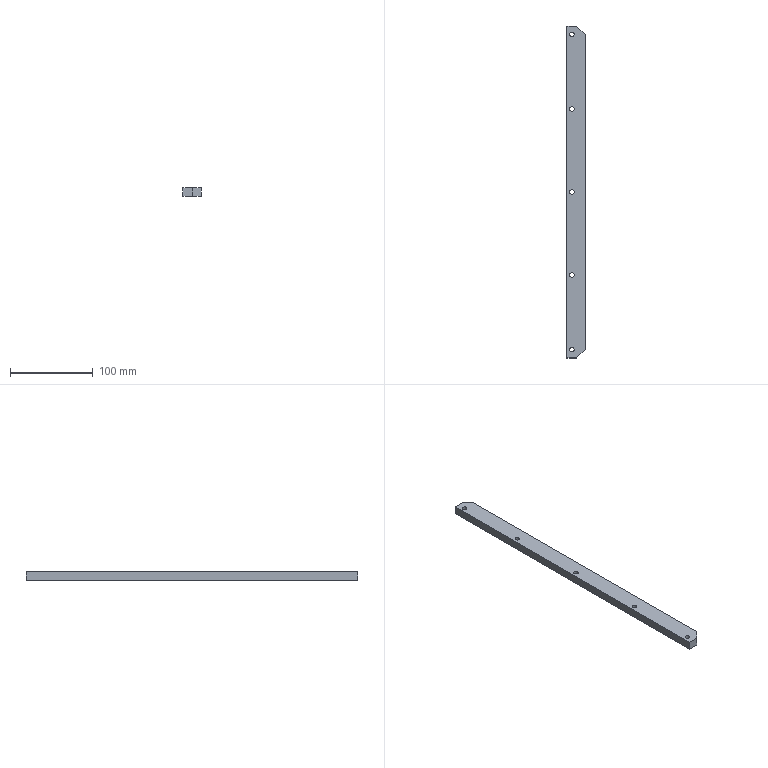Part | STEP file | DSJIN1 | 1 solid | 18 faces | box 22 x 400 x 10 mm | volume 85812 mm3 | cylinder 10 | plane 8 | commonest cylinder face diameters 5.5 x10
STEP:
#1=CARTESIAN_POINT('',(-2.25,100.,10.));
#2=VERTEX_POINT('',#1);
#3=CARTESIAN_POINT('',(-7.75,100.,10.));
#4=VERTEX_POINT('',#3);
#5=CARTESIAN_POINT('',(-5.,100.,10.));
#6=DIRECTION('',(0.,0.,-1.));
#7=DIRECTION('',(-1.,0.,0.));
#8=AXIS2_PLACEMENT_3D('',#5,#6,#7);
#9=CIRCLE('',#8,2.75);
#10=EDGE_CURVE('',#2,#4,#9,.T.);
#11=ORIENTED_EDGE('',*,*,#10,.F.);
#12=CARTESIAN_POINT('',(-2.25,100.,0.));
#13=VERTEX_POINT('',#12);
#14=CARTESIAN_POINT('',(-2.25,100.,0.));
#15=DIRECTION('',(0.,0.,-1.));
#16=VECTOR('',#15,1000.);
#17=LINE('',#14,#16);
#18=EDGE_CURVE('',#2,#13,#17,.T.);
#19=ORIENTED_EDGE('',*,*,#18,.T.);
#20=CARTESIAN_POINT('',(-7.75,100.,0.));
#21=VERTEX_POINT('',#20);
#22=CARTESIAN_POINT('',(-5.,100.,0.));
#23=DIRECTION('',(0.,0.,-1.));
#24=DIRECTION('',(-1.,0.,0.));
#25=AXIS2_PLACEMENT_3D('',#22,#23,#24);
#26=CIRCLE('',#25,2.75);
#27=EDGE_CURVE('',#13,#21,#26,.T.);
#28=ORIENTED_EDGE('',*,*,#27,.T.);
#29=CARTESIAN_POINT('',(-7.75,100.,0.));
#30=DIRECTION('',(0.,0.,-1.));
#31=VECTOR('',#30,1000.);
#32=LINE('',#29,#31);
#33=EDGE_CURVE('',#4,#21,#32,.T.);
#34=ORIENTED_EDGE('',*,*,#33,.F.);
#35=EDGE_LOOP('',(#11,#19,#28,#34));
#36=FACE_OUTER_BOUND('',#35,.T.);
#37=CARTESIAN_POINT('',(-5.,100.,0.));
#38=DIRECTION('',(0.,0.,-1.));
#39=DIRECTION('',(-1.,0.,0.));
#40=AXIS2_PLACEMENT_3D('',#37,#38,#39);
#41=CYLINDRICAL_SURFACE('',#40,2.75);
#42=ADVANCED_FACE('',(#36),#41,.F.);
#43=CARTESIAN_POINT('',(-2.25,0.,10.));
#44=VERTEX_POINT('',#43);
#45=CARTESIAN_POINT('',(-7.75,0.,10.));
#46=VERTEX_POINT('',#45);
#47=CARTESIAN_POINT('',(-5.,0.,10.));
#48=DIRECTION('',(0.,0.,-1.));
#49=DIRECTION('',(-1.,0.,0.));
#50=AXIS2_PLACEMENT_3D('',#47,#48,#49);
#51=CIRCLE('',#50,2.75);
#52=EDGE_CURVE('',#44,#46,#51,.T.);
#53=ORIENTED_EDGE('',*,*,#52,.F.);
#54=CARTESIAN_POINT('',(-2.25,0.,0.));
#55=VERTEX_POINT('',#54);
#56=CARTESIAN_POINT('',(-2.25,0.,0.));
#57=DIRECTION('',(0.,0.,-1.));
#58=VECTOR('',#57,1000.);
#59=LINE('',#56,#58);
#60=EDGE_CURVE('',#44,#55,#59,.T.);
#61=ORIENTED_EDGE('',*,*,#60,.T.);
#62=CARTESIAN_POINT('',(-7.75,0.,0.));
#63=VERTEX_POINT('',#62);
#64=CARTESIAN_POINT('',(-5.,0.,0.));
#65=DIRECTION('',(0.,0.,-1.));
#66=DIRECTION('',(-1.,0.,0.));
#67=AXIS2_PLACEMENT_3D('',#64,#65,#66);
#68=CIRCLE('',#67,2.75);
#69=EDGE_CURVE('',#55,#63,#68,.T.);
#70=ORIENTED_EDGE('',*,*,#69,.T.);
#71=CARTESIAN_POINT('',(-7.75,0.,0.));
#72=DIRECTION('',(0.,0.,-1.));
#73=VECTOR('',#72,1000.);
#74=LINE('',#71,#73);
#75=EDGE_CURVE('',#46,#63,#74,.T.);
#76=ORIENTED_EDGE('',*,*,#75,.F.);
#77=EDGE_LOOP('',(#53,#61,#70,#76));
#78=FACE_OUTER_BOUND('',#77,.T.);
#79=CARTESIAN_POINT('',(-5.,0.,0.));
#80=DIRECTION('',(0.,0.,-1.));
#81=DIRECTION('',(-1.,0.,0.));
#82=AXIS2_PLACEMENT_3D('',#79,#80,#81);
#83=CYLINDRICAL_SURFACE('',#82,2.75);
#84=ADVANCED_FACE('',(#78),#83,.F.);
#85=CARTESIAN_POINT('',(-2.25,-100.,10.));
#86=VERTEX_POINT('',#85);
#87=CARTESIAN_POINT('',(-7.75,-100.,10.));
#88=VERTEX_POINT('',#87);
#89=CARTESIAN_POINT('',(-5.,-100.,10.));
#90=DIRECTION('',(0.,0.,-1.));
#91=DIRECTION('',(-1.,0.,0.));
#92=AXIS2_PLACEMENT_3D('',#89,#90,#91);
#93=CIRCLE('',#92,2.75);
#94=EDGE_CURVE('',#86,#88,#93,.T.);
#95=ORIENTED_EDGE('',*,*,#94,.F.);
#96=CARTESIAN_POINT('',(-2.25,-100.,0.));
#97=VERTEX_POINT('',#96);
#98=CARTESIAN_POINT('',(-2.25,-100.,0.));
#99=DIRECTION('',(0.,0.,-1.));
#100=VECTOR('',#99,1000.);
#101=LINE('',#98,#100);
#102=EDGE_CURVE('',#86,#97,#101,.T.);
#103=ORIENTED_EDGE('',*,*,#102,.T.);
#104=CARTESIAN_POINT('',(-7.75,-100.,0.));
#105=VERTEX_POINT('',#104);
#106=CARTESIAN_POINT('',(-5.,-100.,0.));
#107=DIRECTION('',(0.,0.,-1.));
#108=DIRECTION('',(-1.,0.,0.));
#109=AXIS2_PLACEMENT_3D('',#106,#107,#108);
#110=CIRCLE('',#109,2.75);
#111=EDGE_CURVE('',#97,#105,#110,.T.);
#112=ORIENTED_EDGE('',*,*,#111,.T.);
#113=CARTESIAN_POINT('',(-7.75,-100.,0.));
#114=DIRECTION('',(0.,0.,-1.));
#115=VECTOR('',#114,1000.);
#116=LINE('',#113,#115);
#117=EDGE_CURVE('',#88,#105,#116,.T.);
#118=ORIENTED_EDGE('',*,*,#117,.F.);
#119=EDGE_LOOP('',(#95,#103,#112,#118));
#120=FACE_OUTER_BOUND('',#119,.T.);
#121=CARTESIAN_POINT('',(-5.,-100.,0.));
#122=DIRECTION('',(0.,0.,-1.));
#123=DIRECTION('',(-1.,0.,0.));
#124=AXIS2_PLACEMENT_3D('',#121,#122,#123);
#125=CYLINDRICAL_SURFACE('',#124,2.75);
#126=ADVANCED_FACE('',(#120),#125,.F.);
#127=CARTESIAN_POINT('',(-2.25,-190.,10.));
#128=VERTEX_POINT('',#127);
#129=CARTESIAN_POINT('',(-7.75,-190.,10.));
#130=VERTEX_POINT('',#129);
#131=CARTESIAN_POINT('',(-5.,-190.,10.));
#132=DIRECTION('',(0.,0.,-1.));
#133=DIRECTION('',(-1.,0.,0.));
#134=AXIS2_PLACEMENT_3D('',#131,#132,#133);
#135=CIRCLE('',#134,2.75);
#136=EDGE_CURVE('',#128,#130,#135,.T.);
#137=ORIENTED_EDGE('',*,*,#136,.F.);
#138=CARTESIAN_POINT('',(-2.25,-190.,0.));
#139=VERTEX_POINT('',#138);
#140=CARTESIAN_POINT('',(-2.25,-190.,0.));
#141=DIRECTION('',(0.,0.,-1.));
#142=VECTOR('',#141,1000.);
#143=LINE('',#140,#142);
#144=EDGE_CURVE('',#128,#139,#143,.T.);
#145=ORIENTED_EDGE('',*,*,#144,.T.);
#146=CARTESIAN_POINT('',(-7.75,-190.,0.));
#147=VERTEX_POINT('',#146);
#148=CARTESIAN_POINT('',(-5.,-190.,0.));
#149=DIRECTION('',(0.,0.,-1.));
#150=DIRECTION('',(-1.,0.,0.));
#151=AXIS2_PLACEMENT_3D('',#148,#149,#150);
#152=CIRCLE('',#151,2.75);
#153=EDGE_CURVE('',#139,#147,#152,.T.);
#154=ORIENTED_EDGE('',*,*,#153,.T.);
#155=CARTESIAN_POINT('',(-7.75,-190.,0.));
#156=DIRECTION('',(0.,0.,-1.));
#157=VECTOR('',#156,1000.);
#158=LINE('',#155,#157);
#159=EDGE_CURVE('',#130,#147,#158,.T.);
#160=ORIENTED_EDGE('',*,*,#159,.F.);
#161=EDGE_LOOP('',(#137,#145,#154,#160));
#162=FACE_OUTER_BOUND('',#161,.T.);
#163=CARTESIAN_POINT('',(-5.,-190.,0.));
#164=DIRECTION('',(0.,0.,-1.));
#165=DIRECTION('',(-1.,0.,0.));
#166=AXIS2_PLACEMENT_3D('',#163,#164,#165);
#167=CYLINDRICAL_SURFACE('',#166,2.75);
#168=ADVANCED_FACE('',(#162),#167,.F.);
#169=CARTESIAN_POINT('',(-2.25,190.,10.));
#170=VERTEX_POINT('',#169);
#171=CARTESIAN_POINT('',(-7.75,190.,10.));
#172=VERTEX_POINT('',#171);
#173=CARTESIAN_POINT('',(-5.,190.,10.));
#174=DIRECTION('',(0.,0.,-1.));
#175=DIRECTION('',(-1.,0.,0.));
#176=AXIS2_PLACEMENT_3D('',#173,#174,#175);
#177=CIRCLE('',#176,2.75);
#178=EDGE_CURVE('',#170,#172,#177,.T.);
#179=ORIENTED_EDGE('',*,*,#178,.F.);
#180=CARTESIAN_POINT('',(-2.25,190.,0.));
#181=VERTEX_POINT('',#180);
#182=CARTESIAN_POINT('',(-2.25,190.,0.));
#183=DIRECTION('',(0.,0.,-1.));
#184=VECTOR('',#183,1000.);
#185=LINE('',#182,#184);
#186=EDGE_CURVE('',#170,#181,#185,.T.);
#187=ORIENTED_EDGE('',*,*,#186,.T.);
#188=CARTESIAN_POINT('',(-7.75,190.,0.));
#189=VERTEX_POINT('',#188);
#190=CARTESIAN_POINT('',(-5.,190.,0.));
#191=DIRECTION('',(0.,0.,-1.));
#192=DIRECTION('',(-1.,0.,0.));
#193=AXIS2_PLACEMENT_3D('',#190,#191,#192);
#194=CIRCLE('',#193,2.75);
#195=EDGE_CURVE('',#181,#189,#194,.T.);
#196=ORIENTED_EDGE('',*,*,#195,.T.);
#197=CARTESIAN_POINT('',(-7.75,190.,0.));
#198=DIRECTION('',(0.,0.,-1.));
#199=VECTOR('',#198,1000.);
#200=LINE('',#197,#199);
#201=EDGE_CURVE('',#172,#189,#200,.T.);
#202=ORIENTED_EDGE('',*,*,#201,.F.);
#203=EDGE_LOOP('',(#179,#187,#196,#202));
#204=FACE_OUTER_BOUND('',#203,.T.);
#205=CARTESIAN_POINT('',(-5.,190.,0.));
#206=DIRECTION('',(0.,0.,-1.));
#207=DIRECTION('',(-1.,0.,0.));
#208=AXIS2_PLACEMENT_3D('',#205,#206,#207);
#209=CYLINDRICAL_SURFACE('',#208,2.75);
#210=ADVANCED_FACE('',(#204),#209,.F.);
#211=CARTESIAN_POINT('',(11.,-190.,10.));
#212=VERTEX_POINT('',#211);
#213=CARTESIAN_POINT('',(11.,190.,10.));
#214=VERTEX_POINT('',#213);
#215=CARTESIAN_POINT('',(11.,-200.,10.));
#216=DIRECTION('',(0.,1.,0.));
#217=VECTOR('',#216,1000.);
#218=LINE('',#215,#217);
#219=EDGE_CURVE('',#212,#214,#218,.T.);
#220=ORIENTED_EDGE('',*,*,#219,.F.);
#221=CARTESIAN_POINT('',(11.,-190.,0.));
#222=VERTEX_POINT('',#221);
#223=CARTESIAN_POINT('',(11.,-190.,10.));
#224=DIRECTION('',(0.,0.,-1.));
#225=VECTOR('',#224,1000.);
#226=LINE('',#223,#225);
#227=EDGE_CURVE('',#212,#222,#226,.T.);
#228=ORIENTED_EDGE('',*,*,#227,.T.);
#229=CARTESIAN_POINT('',(11.,190.,0.));
#230=VERTEX_POINT('',#229);
#231=CARTESIAN_POINT('',(11.,-200.,0.));
#232=DIRECTION('',(0.,1.,0.));
#233=VECTOR('',#232,1000.);
#234=LINE('',#231,#233);
#235=EDGE_CURVE('',#222,#230,#234,.T.);
#236=ORIENTED_EDGE('',*,*,#235,.T.);
#237=CARTESIAN_POINT('',(11.,190.,10.));
#238=DIRECTION('',(0.,0.,1.));
#239=VECTOR('',#238,1000.);
#240=LINE('',#237,#239);
#241=EDGE_CURVE('',#230,#214,#240,.T.);
#242=ORIENTED_EDGE('',*,*,#241,.T.);
#243=EDGE_LOOP('',(#220,#228,#236,#242));
#244=FACE_OUTER_BOUND('',#243,.T.);
#245=CARTESIAN_POINT('',(11.,-200.,10.));
#246=DIRECTION('',(-1.,0.,0.));
#247=DIRECTION('',(0.,0.,1.));
#248=AXIS2_PLACEMENT_3D('',#245,#246,#247);
#249=PLANE('',#248);
#250=ADVANCED_FACE('',(#244),#249,.F.);
#251=CARTESIAN_POINT('',(1.,200.,10.));
#252=VERTEX_POINT('',#251);
#253=CARTESIAN_POINT('',(-11.,200.,10.));
#254=VERTEX_POINT('',#253);
#255=CARTESIAN_POINT('',(-11.,200.,10.));
#256=DIRECTION('',(-1.,0.,0.));
#257=VECTOR('',#256,1000.);
#258=LINE('',#255,#257);
#259=EDGE_CURVE('',#252,#254,#258,.T.);
#260=ORIENTED_EDGE('',*,*,#259,.F.);
#261=CARTESIAN_POINT('',(1.,200.,0.));
#262=VERTEX_POINT('',#261);
#263=CARTESIAN_POINT('',(1.,200.,10.));
#264=DIRECTION('',(0.,0.,-1.));
#265=VECTOR('',#264,1000.);
#266=LINE('',#263,#265);
#267=EDGE_CURVE('',#252,#262,#266,.T.);
#268=ORIENTED_EDGE('',*,*,#267,.T.);
#269=CARTESIAN_POINT('',(-11.,200.,0.));
#270=VERTEX_POINT('',#269);
#271=CARTESIAN_POINT('',(-11.,200.,0.));
#272=DIRECTION('',(-1.,0.,0.));
#273=VECTOR('',#272,1000.);
#274=LINE('',#271,#273);
#275=EDGE_CURVE('',#262,#270,#274,.T.);
#276=ORIENTED_EDGE('',*,*,#275,.T.);
#277=CARTESIAN_POINT('',(-11.,200.,10.));
#278=DIRECTION('',(0.,0.,-1.));
#279=VECTOR('',#278,1000.);
#280=LINE('',#277,#279);
#281=EDGE_CURVE('',#254,#270,#280,.T.);
#282=ORIENTED_EDGE('',*,*,#281,.F.);
#283=EDGE_LOOP('',(#260,#268,#276,#282));
#284=FACE_OUTER_BOUND('',#283,.T.);
#285=CARTESIAN_POINT('',(-11.,200.,10.));
#286=DIRECTION('',(0.,-1.,0.));
#287=DIRECTION('',(0.,0.,-1.));
#288=AXIS2_PLACEMENT_3D('',#285,#286,#287);
#289=PLANE('',#288);
#290=ADVANCED_FACE('',(#284),#289,.F.);
#291=CARTESIAN_POINT('',(-11.,-200.,0.));
#292=VERTEX_POINT('',#291);
#293=CARTESIAN_POINT('',(-11.,-200.,0.));
#294=DIRECTION('',(0.,-1.,0.));
#295=VECTOR('',#294,1000.);
#296=LINE('',#293,#295);
#297=EDGE_CURVE('',#270,#292,#296,.T.);
#298=ORIENTED_EDGE('',*,*,#297,.T.);
#299=CARTESIAN_POINT('',(-11.,-200.,10.));
#300=VERTEX_POINT('',#299);
#301=CARTESIAN_POINT('',(-11.,-200.,10.));
#302=DIRECTION('',(0.,0.,-1.));
#303=VECTOR('',#302,1000.);
#304=LINE('',#301,#303);
#305=EDGE_CURVE('',#300,#292,#304,.T.);
#306=ORIENTED_EDGE('',*,*,#305,.F.);
#307=CARTESIAN_POINT('',(-11.,-200.,10.));
#308=DIRECTION('',(0.,-1.,0.));
#309=VECTOR('',#308,1000.);
#310=LINE('',#307,#309);
#311=EDGE_CURVE('',#254,#300,#310,.T.);
#312=ORIENTED_EDGE('',*,*,#311,.F.);
#313=ORIENTED_EDGE('',*,*,#281,.T.);
#314=EDGE_LOOP('',(#298,#306,#312,#313));
#315=FACE_OUTER_BOUND('',#314,.T.);
#316=CARTESIAN_POINT('',(-11.,-200.,10.));
#317=DIRECTION('',(1.,0.,0.));
#318=DIRECTION('',(0.,0.,-1.));
#319=AXIS2_PLACEMENT_3D('',#316,#317,#318);
#320=PLANE('',#319);
#321=ADVANCED_FACE('',(#315),#320,.F.);
#322=CARTESIAN_POINT('',(1.,-200.,0.));
#323=VERTEX_POINT('',#322);
#324=CARTESIAN_POINT('',(-11.,-200.,0.));
#325=DIRECTION('',(1.,0.,0.));
#326=VECTOR('',#325,1000.);
#327=LINE('',#324,#326);
#328=EDGE_CURVE('',#292,#323,#327,.T.);
#329=ORIENTED_EDGE('',*,*,#328,.T.);
#330=CARTESIAN_POINT('',(1.,-200.,10.));
#331=VERTEX_POINT('',#330);
#332=CARTESIAN_POINT('',(1.,-200.,10.));
#333=DIRECTION('',(0.,0.,1.));
#334=VECTOR('',#333,1000.);
#335=LINE('',#332,#334);
#336=EDGE_CURVE('',#323,#331,#335,.T.);
#337=ORIENTED_EDGE('',*,*,#336,.T.);
#338=CARTESIAN_POINT('',(-11.,-200.,10.));
#339=DIRECTION('',(1.,0.,0.));
#340=VECTOR('',#339,1000.);
#341=LINE('',#338,#340);
#342=EDGE_CURVE('',#300,#331,#341,.T.);
#343=ORIENTED_EDGE('',*,*,#342,.F.);
#344=ORIENTED_EDGE('',*,*,#305,.T.);
#345=EDGE_LOOP('',(#329,#337,#343,#344));
#346=FACE_OUTER_BOUND('',#345,.T.);
#347=CARTESIAN_POINT('',(-11.,-200.,10.));
#348=DIRECTION('',(0.,1.,0.));
#349=DIRECTION('',(0.,0.,1.));
#350=AXIS2_PLACEMENT_3D('',#347,#348,#349);
#351=PLANE('',#350);
#352=ADVANCED_FACE('',(#346),#351,.F.);
#353=CARTESIAN_POINT('',(-5.,100.,10.));
#354=DIRECTION('',(0.,0.,-1.));
#355=DIRECTION('',(-1.,0.,0.));
#356=AXIS2_PLACEMENT_3D('',#353,#354,#355);
#357=CIRCLE('',#356,2.75);
#358=EDGE_CURVE('',#4,#2,#357,.T.);
#359=ORIENTED_EDGE('',*,*,#358,.T.);
#360=ORIENTED_EDGE('',*,*,#10,.T.);
#361=EDGE_LOOP('',(#359,#360));
#362=FACE_BOUND('',#361,.T.);
#363=CARTESIAN_POINT('',(-5.,0.,10.));
#364=DIRECTION('',(0.,0.,-1.));
#365=DIRECTION('',(-1.,0.,0.));
#366=AXIS2_PLACEMENT_3D('',#363,#364,#365);
#367=CIRCLE('',#366,2.75);
#368=EDGE_CURVE('',#46,#44,#367,.T.);
#369=ORIENTED_EDGE('',*,*,#368,.T.);
#370=ORIENTED_EDGE('',*,*,#52,.T.);
#371=EDGE_LOOP('',(#369,#370));
#372=FACE_BOUND('',#371,.T.);
#373=CARTESIAN_POINT('',(-5.,-100.,10.));
#374=DIRECTION('',(0.,0.,-1.));
#375=DIRECTION('',(-1.,0.,0.));
#376=AXIS2_PLACEMENT_3D('',#373,#374,#375);
#377=CIRCLE('',#376,2.75);
#378=EDGE_CURVE('',#88,#86,#377,.T.);
#379=ORIENTED_EDGE('',*,*,#378,.T.);
#380=ORIENTED_EDGE('',*,*,#94,.T.);
#381=EDGE_LOOP('',(#379,#380));
#382=FACE_BOUND('',#381,.T.);
#383=CARTESIAN_POINT('',(-5.,-190.,10.));
#384=DIRECTION('',(0.,0.,-1.));
#385=DIRECTION('',(-1.,0.,0.));
#386=AXIS2_PLACEMENT_3D('',#383,#384,#385);
#387=CIRCLE('',#386,2.75);
#388=EDGE_CURVE('',#130,#128,#387,.T.);
#389=ORIENTED_EDGE('',*,*,#388,.T.);
#390=ORIENTED_EDGE('',*,*,#136,.T.);
#391=EDGE_LOOP('',(#389,#390));
#392=FACE_BOUND('',#391,.T.);
#393=CARTESIAN_POINT('',(-5.,190.,10.));
#394=DIRECTION('',(0.,0.,-1.));
#395=DIRECTION('',(-1.,0.,0.));
#396=AXIS2_PLACEMENT_3D('',#393,#394,#395);
#397=CIRCLE('',#396,2.75);
#398=EDGE_CURVE('',#172,#170,#397,.T.);
#399=ORIENTED_EDGE('',*,*,#398,.T.);
#400=ORIENTED_EDGE('',*,*,#178,.T.);
#401=EDGE_LOOP('',(#399,#400));
#402=FACE_BOUND('',#401,.T.);
#403=ORIENTED_EDGE('',*,*,#342,.T.);
#404=CARTESIAN_POINT('',(11.,-190.,10.));
#405=DIRECTION('',(0.7071,0.7071,0.));
#406=VECTOR('',#405,1000.);
#407=LINE('',#404,#406);
#408=EDGE_CURVE('',#331,#212,#407,.T.);
#409=ORIENTED_EDGE('',*,*,#408,.T.);
#410=ORIENTED_EDGE('',*,*,#219,.T.);
#411=CARTESIAN_POINT('',(1.,200.,10.));
#412=DIRECTION('',(-0.7071,0.7071,0.));
#413=VECTOR('',#412,1000.);
#414=LINE('',#411,#413);
#415=EDGE_CURVE('',#214,#252,#414,.T.);
#416=ORIENTED_EDGE('',*,*,#415,.T.);
#417=ORIENTED_EDGE('',*,*,#259,.T.);
#418=ORIENTED_EDGE('',*,*,#311,.T.);
#419=EDGE_LOOP('',(#403,#409,#410,#416,#417,#418));
#420=FACE_OUTER_BOUND('',#419,.T.);
#421=CARTESIAN_POINT('',(0.,0.,10.));
#422=DIRECTION('',(0.,0.,-1.));
#423=DIRECTION('',(-1.,0.,0.));
#424=AXIS2_PLACEMENT_3D('',#421,#422,#423);
#425=PLANE('',#424);
#426=ADVANCED_FACE('',(#362,#372,#382,#392,#402,#420),#425,.F.);
#427=CARTESIAN_POINT('',(-5.,100.,0.));
#428=DIRECTION('',(0.,0.,-1.));
#429=DIRECTION('',(-1.,0.,0.));
#430=AXIS2_PLACEMENT_3D('',#427,#428,#429);
#431=CIRCLE('',#430,2.75);
#432=EDGE_CURVE('',#21,#13,#431,.T.);
#433=ORIENTED_EDGE('',*,*,#432,.F.);
#434=ORIENTED_EDGE('',*,*,#27,.F.);
#435=EDGE_LOOP('',(#433,#434));
#436=FACE_BOUND('',#435,.T.);
#437=CARTESIAN_POINT('',(-5.,0.,0.));
#438=DIRECTION('',(0.,0.,-1.));
#439=DIRECTION('',(-1.,0.,0.));
#440=AXIS2_PLACEMENT_3D('',#437,#438,#439);
#441=CIRCLE('',#440,2.75);
#442=EDGE_CURVE('',#63,#55,#441,.T.);
#443=ORIENTED_EDGE('',*,*,#442,.F.);
#444=ORIENTED_EDGE('',*,*,#69,.F.);
#445=EDGE_LOOP('',(#443,#444));
#446=FACE_BOUND('',#445,.T.);
#447=CARTESIAN_POINT('',(-5.,-100.,0.));
#448=DIRECTION('',(0.,0.,-1.));
#449=DIRECTION('',(-1.,0.,0.));
#450=AXIS2_PLACEMENT_3D('',#447,#448,#449);
#451=CIRCLE('',#450,2.75);
#452=EDGE_CURVE('',#105,#97,#451,.T.);
#453=ORIENTED_EDGE('',*,*,#452,.F.);
#454=ORIENTED_EDGE('',*,*,#111,.F.);
#455=EDGE_LOOP('',(#453,#454));
#456=FACE_BOUND('',#455,.T.);
#457=CARTESIAN_POINT('',(-5.,-190.,0.));
#458=DIRECTION('',(0.,0.,-1.));
#459=DIRECTION('',(-1.,0.,0.));
#460=AXIS2_PLACEMENT_3D('',#457,#458,#459);
#461=CIRCLE('',#460,2.75);
#462=EDGE_CURVE('',#147,#139,#461,.T.);
#463=ORIENTED_EDGE('',*,*,#462,.F.);
#464=ORIENTED_EDGE('',*,*,#153,.F.);
#465=EDGE_LOOP('',(#463,#464));
#466=FACE_BOUND('',#465,.T.);
#467=CARTESIAN_POINT('',(-5.,190.,0.));
#468=DIRECTION('',(0.,0.,-1.));
#469=DIRECTION('',(-1.,0.,0.));
#470=AXIS2_PLACEMENT_3D('',#467,#468,#469);
#471=CIRCLE('',#470,2.75);
#472=EDGE_CURVE('',#189,#181,#471,.T.);
#473=ORIENTED_EDGE('',*,*,#472,.F.);
#474=ORIENTED_EDGE('',*,*,#195,.F.);
#475=EDGE_LOOP('',(#473,#474));
#476=FACE_BOUND('',#475,.T.);
#477=ORIENTED_EDGE('',*,*,#235,.F.);
#478=CARTESIAN_POINT('',(100.5,-100.5,0.));
#479=DIRECTION('',(-0.7071,-0.7071,0.));
#480=VECTOR('',#479,1000.);
#481=LINE('',#478,#480);
#482=EDGE_CURVE('',#222,#323,#481,.T.);
#483=ORIENTED_EDGE('',*,*,#482,.T.);
#484=ORIENTED_EDGE('',*,*,#328,.F.);
#485=ORIENTED_EDGE('',*,*,#297,.F.);
#486=ORIENTED_EDGE('',*,*,#275,.F.);
#487=CARTESIAN_POINT('',(100.5,100.5,0.));
#488=DIRECTION('',(0.7071,-0.7071,0.));
#489=VECTOR('',#488,1000.);
#490=LINE('',#487,#489);
#491=EDGE_CURVE('',#262,#230,#490,.T.);
#492=ORIENTED_EDGE('',*,*,#491,.T.);
#493=EDGE_LOOP('',(#477,#483,#484,#485,#486,#492));
#494=FACE_OUTER_BOUND('',#493,.T.);
#495=CARTESIAN_POINT('',(0.,0.,0.));
#496=DIRECTION('',(0.,0.,-1.));
#497=DIRECTION('',(-1.,0.,0.));
#498=AXIS2_PLACEMENT_3D('',#495,#496,#497);
#499=PLANE('',#498);
#500=ADVANCED_FACE('',(#436,#446,#456,#466,#476,#494),#499,.T.);
#501=ORIENTED_EDGE('',*,*,#186,.F.);
#502=ORIENTED_EDGE('',*,*,#398,.F.);
#503=ORIENTED_EDGE('',*,*,#201,.T.);
#504=ORIENTED_EDGE('',*,*,#472,.T.);
#505=EDGE_LOOP('',(#501,#502,#503,#504));
#506=FACE_OUTER_BOUND('',#505,.T.);
#507=CARTESIAN_POINT('',(-5.,190.,0.));
#508=DIRECTION('',(0.,0.,-1.));
#509=DIRECTION('',(-1.,0.,0.));
#510=AXIS2_PLACEMENT_3D('',#507,#508,#509);
#511=CYLINDRICAL_SURFACE('',#510,2.75);
#512=ADVANCED_FACE('',(#506),#511,.F.);
#513=ORIENTED_EDGE('',*,*,#144,.F.);
#514=ORIENTED_EDGE('',*,*,#388,.F.);
#515=ORIENTED_EDGE('',*,*,#159,.T.);
#516=ORIENTED_EDGE('',*,*,#462,.T.);
#517=EDGE_LOOP('',(#513,#514,#515,#516));
#518=FACE_OUTER_BOUND('',#517,.T.);
#519=CARTESIAN_POINT('',(-5.,-190.,0.));
#520=DIRECTION('',(0.,0.,-1.));
#521=DIRECTION('',(-1.,0.,0.));
#522=AXIS2_PLACEMENT_3D('',#519,#520,#521);
#523=CYLINDRICAL_SURFACE('',#522,2.75);
#524=ADVANCED_FACE('',(#518),#523,.F.);
#525=ORIENTED_EDGE('',*,*,#102,.F.);
#526=ORIENTED_EDGE('',*,*,#378,.F.);
#527=ORIENTED_EDGE('',*,*,#117,.T.);
#528=ORIENTED_EDGE('',*,*,#452,.T.);
#529=EDGE_LOOP('',(#525,#526,#527,#528));
#530=FACE_OUTER_BOUND('',#529,.T.);
#531=CARTESIAN_POINT('',(-5.,-100.,0.));
#532=DIRECTION('',(0.,0.,-1.));
#533=DIRECTION('',(-1.,0.,0.));
#534=AXIS2_PLACEMENT_3D('',#531,#532,#533);
#535=CYLINDRICAL_SURFACE('',#534,2.75);
#536=ADVANCED_FACE('',(#530),#535,.F.);
#537=ORIENTED_EDGE('',*,*,#60,.F.);
#538=ORIENTED_EDGE('',*,*,#368,.F.);
#539=ORIENTED_EDGE('',*,*,#75,.T.);
#540=ORIENTED_EDGE('',*,*,#442,.T.);
#541=EDGE_LOOP('',(#537,#538,#539,#540));
#542=FACE_OUTER_BOUND('',#541,.T.);
#543=CARTESIAN_POINT('',(-5.,0.,0.));
#544=DIRECTION('',(0.,0.,-1.));
#545=DIRECTION('',(-1.,0.,0.));
#546=AXIS2_PLACEMENT_3D('',#543,#544,#545);
#547=CYLINDRICAL_SURFACE('',#546,2.75);
#548=ADVANCED_FACE('',(#542),#547,.F.);
#549=ORIENTED_EDGE('',*,*,#18,.F.);
#550=ORIENTED_EDGE('',*,*,#358,.F.);
#551=ORIENTED_EDGE('',*,*,#33,.T.);
#552=ORIENTED_EDGE('',*,*,#432,.T.);
#553=EDGE_LOOP('',(#549,#550,#551,#552));
#554=FACE_OUTER_BOUND('',#553,.T.);
#555=CARTESIAN_POINT('',(-5.,100.,0.));
#556=DIRECTION('',(0.,0.,-1.));
#557=DIRECTION('',(-1.,0.,0.));
#558=AXIS2_PLACEMENT_3D('',#555,#556,#557);
#559=CYLINDRICAL_SURFACE('',#558,2.75);
#560=ADVANCED_FACE('',(#554),#559,.F.);
#561=ORIENTED_EDGE('',*,*,#408,.F.);
#562=ORIENTED_EDGE('',*,*,#336,.F.);
#563=ORIENTED_EDGE('',*,*,#482,.F.);
#564=ORIENTED_EDGE('',*,*,#227,.F.);
#565=EDGE_LOOP('',(#561,#562,#563,#564));
#566=FACE_OUTER_BOUND('',#565,.T.);
#567=CARTESIAN_POINT('',(11.,-190.,10.));
#568=DIRECTION('',(-0.7071,0.7071,0.));
#569=DIRECTION('',(0.,0.,-1.));
#570=AXIS2_PLACEMENT_3D('',#567,#568,#569);
#571=PLANE('',#570);
#572=ADVANCED_FACE('',(#566),#571,.F.);
#573=ORIENTED_EDGE('',*,*,#415,.F.);
#574=ORIENTED_EDGE('',*,*,#241,.F.);
#575=ORIENTED_EDGE('',*,*,#491,.F.);
#576=ORIENTED_EDGE('',*,*,#267,.F.);
#577=EDGE_LOOP('',(#573,#574,#575,#576));
#578=FACE_OUTER_BOUND('',#577,.T.);
#579=CARTESIAN_POINT('',(1.,200.,10.));
#580=DIRECTION('',(-0.7071,-0.7071,0.));
#581=DIRECTION('',(0.,0.,-1.));
#582=AXIS2_PLACEMENT_3D('',#579,#580,#581);
#583=PLANE('',#582);
#584=ADVANCED_FACE('',(#578),#583,.F.);
#585=CLOSED_SHELL('',(#42,#84,#126,#168,#210,#250,#290,#321,#352,#426,#500,#512,#524,#536,#548,#560,#572,#584));
#586=MANIFOLD_SOLID_BREP('',#585);
#587=CARTESIAN_POINT('',(0.,0.,0.));
#588=DIRECTION('',(0.,0.,1.));
#589=DIRECTION('',(1.,0.,0.));
#590=AXIS2_PLACEMENT_3D('',#587,#588,#589);
#591=(LENGTH_UNIT()NAMED_UNIT(*)SI_UNIT(.MILLI.,.METRE.));
#592=UNCERTAINTY_MEASURE_WITH_UNIT(LENGTH_MEASURE(0.00001),#591,'','');
#593=(NAMED_UNIT(*)PLANE_ANGLE_UNIT()SI_UNIT($,.RADIAN.));
#594=(NAMED_UNIT(*)SI_UNIT($,.STERADIAN.)SOLID_ANGLE_UNIT());
#595=(GEOMETRIC_REPRESENTATION_CONTEXT(3)GLOBAL_UNCERTAINTY_ASSIGNED_CONTEXT((#592))GLOBAL_UNIT_ASSIGNED_CONTEXT((#591,#593,#594))REPRESENTATION_CONTEXT('',''));
#596=ADVANCED_BREP_SHAPE_REPRESENTATION('',(#586,#590),#595);